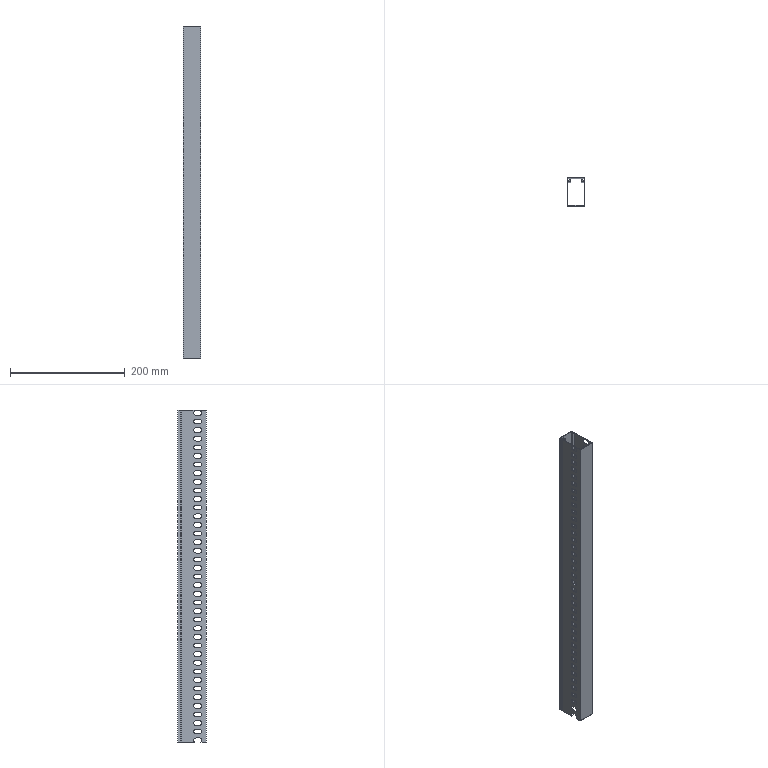Part | SolidWorks | features BaseBody 1 | 1 solid | 337 faces | box 30 x 50 x 578 mm | volume 94083 mm3 | plane 181 | cylinder 156 | commonest cylinder face diameters 8 x156